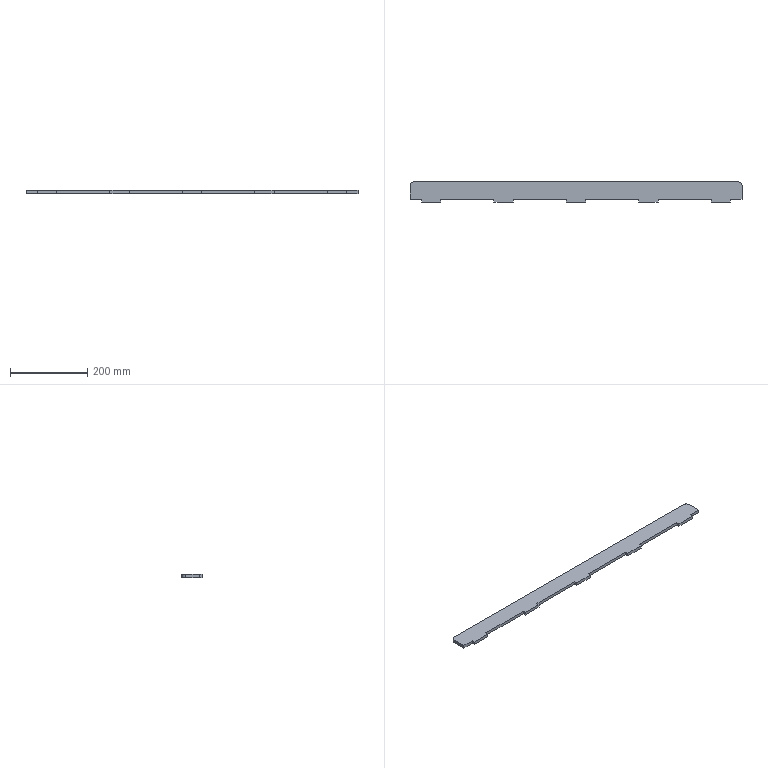Part | SolidWorks | features FlatPattern 1, SMBaseFlange 1, SheetMetal 1 | 1 solid | 28 faces | box 860 x 52.5 x 8 mm | volume 324257 mm3 | plane 26 | cylinder 2 | commonest cylinder face diameters 20 x2
STEP:
#1=CARTESIAN_POINT('',(438.717,-866.,0.));
#2=VERTEX_POINT('',#1);
#3=CARTESIAN_POINT('',(438.717,-831.,0.));
#4=VERTEX_POINT('',#3);
#5=CARTESIAN_POINT('',(438.717,-866.,0.));
#6=DIRECTION('',(0.,1.,0.));
#7=VECTOR('',#6,1000.);
#8=LINE('',#5,#7);
#9=EDGE_CURVE('',#2,#4,#8,.T.);
#10=ORIENTED_EDGE('',*,*,#9,.F.);
#11=CARTESIAN_POINT('',(438.717,-866.,-8.));
#12=VERTEX_POINT('',#11);
#13=CARTESIAN_POINT('',(438.717,-866.,-8.));
#14=DIRECTION('',(0.,0.,1.));
#15=VECTOR('',#14,1000.);
#16=LINE('',#13,#15);
#17=EDGE_CURVE('',#12,#2,#16,.T.);
#18=ORIENTED_EDGE('',*,*,#17,.F.);
#19=CARTESIAN_POINT('',(438.717,-831.,-8.));
#20=VERTEX_POINT('',#19);
#21=CARTESIAN_POINT('',(438.717,-866.,-8.));
#22=DIRECTION('',(0.,1.,0.));
#23=VECTOR('',#22,1000.);
#24=LINE('',#21,#23);
#25=EDGE_CURVE('',#12,#20,#24,.T.);
#26=ORIENTED_EDGE('',*,*,#25,.T.);
#27=CARTESIAN_POINT('',(438.717,-831.,-8.));
#28=DIRECTION('',(0.,0.,1.));
#29=VECTOR('',#28,1000.);
#30=LINE('',#27,#29);
#31=EDGE_CURVE('',#20,#4,#30,.T.);
#32=ORIENTED_EDGE('',*,*,#31,.T.);
#33=EDGE_LOOP('',(#10,#18,#26,#32));
#34=FACE_OUTER_BOUND('',#33,.T.);
#35=CARTESIAN_POINT('',(438.717,-866.,-8.));
#36=DIRECTION('',(1.,0.,0.));
#37=DIRECTION('',(0.,0.,-1.));
#38=AXIS2_PLACEMENT_3D('',#35,#36,#37);
#39=PLANE('',#38);
#40=ADVANCED_FACE('',(#34),#39,.T.);
#41=CARTESIAN_POINT('',(408.717,-866.,0.));
#42=VERTEX_POINT('',#41);
#43=CARTESIAN_POINT('',(438.717,-866.,0.));
#44=DIRECTION('',(1.,0.,0.));
#45=VECTOR('',#44,1000.);
#46=LINE('',#43,#45);
#47=EDGE_CURVE('',#42,#2,#46,.T.);
#48=ORIENTED_EDGE('',*,*,#47,.F.);
#49=CARTESIAN_POINT('',(408.717,-866.,-8.));
#50=VERTEX_POINT('',#49);
#51=CARTESIAN_POINT('',(408.717,-866.,-8.));
#52=DIRECTION('',(0.,0.,1.));
#53=VECTOR('',#52,1000.);
#54=LINE('',#51,#53);
#55=EDGE_CURVE('',#50,#42,#54,.T.);
#56=ORIENTED_EDGE('',*,*,#55,.F.);
#57=CARTESIAN_POINT('',(438.717,-866.,-8.));
#58=DIRECTION('',(1.,0.,0.));
#59=VECTOR('',#58,1000.);
#60=LINE('',#57,#59);
#61=EDGE_CURVE('',#50,#12,#60,.T.);
#62=ORIENTED_EDGE('',*,*,#61,.T.);
#63=ORIENTED_EDGE('',*,*,#17,.T.);
#64=EDGE_LOOP('',(#48,#56,#62,#63));
#65=FACE_OUTER_BOUND('',#64,.T.);
#66=CARTESIAN_POINT('',(438.717,-866.,-8.));
#67=DIRECTION('',(0.,-1.,0.));
#68=DIRECTION('',(0.,0.,-1.));
#69=AXIS2_PLACEMENT_3D('',#66,#67,#68);
#70=PLANE('',#69);
#71=ADVANCED_FACE('',(#65),#70,.T.);
#72=CARTESIAN_POINT('',(408.717,-873.5,0.));
#73=VERTEX_POINT('',#72);
#74=CARTESIAN_POINT('',(408.717,-866.,0.));
#75=DIRECTION('',(0.,1.,0.));
#76=VECTOR('',#75,1000.);
#77=LINE('',#74,#76);
#78=EDGE_CURVE('',#73,#42,#77,.T.);
#79=ORIENTED_EDGE('',*,*,#78,.F.);
#80=CARTESIAN_POINT('',(408.717,-873.5,-8.));
#81=VERTEX_POINT('',#80);
#82=CARTESIAN_POINT('',(408.717,-873.5,-8.));
#83=DIRECTION('',(0.,0.,1.));
#84=VECTOR('',#83,1000.);
#85=LINE('',#82,#84);
#86=EDGE_CURVE('',#81,#73,#85,.T.);
#87=ORIENTED_EDGE('',*,*,#86,.F.);
#88=CARTESIAN_POINT('',(408.717,-866.,-8.));
#89=DIRECTION('',(0.,1.,0.));
#90=VECTOR('',#89,1000.);
#91=LINE('',#88,#90);
#92=EDGE_CURVE('',#81,#50,#91,.T.);
#93=ORIENTED_EDGE('',*,*,#92,.T.);
#94=ORIENTED_EDGE('',*,*,#55,.T.);
#95=EDGE_LOOP('',(#79,#87,#93,#94));
#96=FACE_OUTER_BOUND('',#95,.T.);
#97=CARTESIAN_POINT('',(408.717,-866.,-8.));
#98=DIRECTION('',(1.,0.,0.));
#99=DIRECTION('',(0.,0.,-1.));
#100=AXIS2_PLACEMENT_3D('',#97,#98,#99);
#101=PLANE('',#100);
#102=ADVANCED_FACE('',(#96),#101,.T.);
#103=CARTESIAN_POINT('',(358.717,-873.5,0.));
#104=VERTEX_POINT('',#103);
#105=CARTESIAN_POINT('',(408.717,-873.5,0.));
#106=DIRECTION('',(1.,0.,0.));
#107=VECTOR('',#106,1000.);
#108=LINE('',#105,#107);
#109=EDGE_CURVE('',#104,#73,#108,.T.);
#110=ORIENTED_EDGE('',*,*,#109,.F.);
#111=CARTESIAN_POINT('',(358.717,-873.5,-8.));
#112=VERTEX_POINT('',#111);
#113=CARTESIAN_POINT('',(358.717,-873.5,-8.));
#114=DIRECTION('',(0.,0.,1.));
#115=VECTOR('',#114,1000.);
#116=LINE('',#113,#115);
#117=EDGE_CURVE('',#112,#104,#116,.T.);
#118=ORIENTED_EDGE('',*,*,#117,.F.);
#119=CARTESIAN_POINT('',(408.717,-873.5,-8.));
#120=DIRECTION('',(1.,0.,0.));
#121=VECTOR('',#120,1000.);
#122=LINE('',#119,#121);
#123=EDGE_CURVE('',#112,#81,#122,.T.);
#124=ORIENTED_EDGE('',*,*,#123,.T.);
#125=ORIENTED_EDGE('',*,*,#86,.T.);
#126=EDGE_LOOP('',(#110,#118,#124,#125));
#127=FACE_OUTER_BOUND('',#126,.T.);
#128=CARTESIAN_POINT('',(408.717,-873.5,-8.));
#129=DIRECTION('',(0.,-1.,0.));
#130=DIRECTION('',(0.,0.,-1.));
#131=AXIS2_PLACEMENT_3D('',#128,#129,#130);
#132=PLANE('',#131);
#133=ADVANCED_FACE('',(#127),#132,.T.);
#134=CARTESIAN_POINT('',(358.717,-866.,0.));
#135=VERTEX_POINT('',#134);
#136=CARTESIAN_POINT('',(358.717,-873.5,0.));
#137=DIRECTION('',(0.,-1.,0.));
#138=VECTOR('',#137,1000.);
#139=LINE('',#136,#138);
#140=EDGE_CURVE('',#135,#104,#139,.T.);
#141=ORIENTED_EDGE('',*,*,#140,.F.);
#142=CARTESIAN_POINT('',(358.717,-866.,-8.));
#143=VERTEX_POINT('',#142);
#144=CARTESIAN_POINT('',(358.717,-866.,-8.));
#145=DIRECTION('',(0.,0.,1.));
#146=VECTOR('',#145,1000.);
#147=LINE('',#144,#146);
#148=EDGE_CURVE('',#143,#135,#147,.T.);
#149=ORIENTED_EDGE('',*,*,#148,.F.);
#150=CARTESIAN_POINT('',(358.717,-873.5,-8.));
#151=DIRECTION('',(0.,-1.,0.));
#152=VECTOR('',#151,1000.);
#153=LINE('',#150,#152);
#154=EDGE_CURVE('',#143,#112,#153,.T.);
#155=ORIENTED_EDGE('',*,*,#154,.T.);
#156=ORIENTED_EDGE('',*,*,#117,.T.);
#157=EDGE_LOOP('',(#141,#149,#155,#156));
#158=FACE_OUTER_BOUND('',#157,.T.);
#159=CARTESIAN_POINT('',(358.717,-873.5,-8.));
#160=DIRECTION('',(-1.,0.,0.));
#161=DIRECTION('',(0.,0.,1.));
#162=AXIS2_PLACEMENT_3D('',#159,#160,#161);
#163=PLANE('',#162);
#164=ADVANCED_FACE('',(#158),#163,.T.);
#165=CARTESIAN_POINT('',(221.217,-866.,0.));
#166=VERTEX_POINT('',#165);
#167=CARTESIAN_POINT('',(358.717,-866.,0.));
#168=DIRECTION('',(1.,0.,0.));
#169=VECTOR('',#168,1000.);
#170=LINE('',#167,#169);
#171=EDGE_CURVE('',#166,#135,#170,.T.);
#172=ORIENTED_EDGE('',*,*,#171,.F.);
#173=CARTESIAN_POINT('',(221.217,-866.,-8.));
#174=VERTEX_POINT('',#173);
#175=CARTESIAN_POINT('',(221.217,-866.,-8.));
#176=DIRECTION('',(0.,0.,1.));
#177=VECTOR('',#176,1000.);
#178=LINE('',#175,#177);
#179=EDGE_CURVE('',#174,#166,#178,.T.);
#180=ORIENTED_EDGE('',*,*,#179,.F.);
#181=CARTESIAN_POINT('',(358.717,-866.,-8.));
#182=DIRECTION('',(1.,0.,0.));
#183=VECTOR('',#182,1000.);
#184=LINE('',#181,#183);
#185=EDGE_CURVE('',#174,#143,#184,.T.);
#186=ORIENTED_EDGE('',*,*,#185,.T.);
#187=ORIENTED_EDGE('',*,*,#148,.T.);
#188=EDGE_LOOP('',(#172,#180,#186,#187));
#189=FACE_OUTER_BOUND('',#188,.T.);
#190=CARTESIAN_POINT('',(358.717,-866.,-8.));
#191=DIRECTION('',(0.,-1.,0.));
#192=DIRECTION('',(1.,0.,0.));
#193=AXIS2_PLACEMENT_3D('',#190,#191,#192);
#194=PLANE('',#193);
#195=ADVANCED_FACE('',(#189),#194,.T.);
#196=CARTESIAN_POINT('',(221.217,-873.5,0.));
#197=VERTEX_POINT('',#196);
#198=CARTESIAN_POINT('',(221.217,-866.,0.));
#199=DIRECTION('',(0.,1.,0.));
#200=VECTOR('',#199,1000.);
#201=LINE('',#198,#200);
#202=EDGE_CURVE('',#197,#166,#201,.T.);
#203=ORIENTED_EDGE('',*,*,#202,.F.);
#204=CARTESIAN_POINT('',(221.217,-873.5,-8.));
#205=VERTEX_POINT('',#204);
#206=CARTESIAN_POINT('',(221.217,-873.5,-8.));
#207=DIRECTION('',(0.,0.,1.));
#208=VECTOR('',#207,1000.);
#209=LINE('',#206,#208);
#210=EDGE_CURVE('',#205,#197,#209,.T.);
#211=ORIENTED_EDGE('',*,*,#210,.F.);
#212=CARTESIAN_POINT('',(221.217,-866.,-8.));
#213=DIRECTION('',(0.,1.,0.));
#214=VECTOR('',#213,1000.);
#215=LINE('',#212,#214);
#216=EDGE_CURVE('',#205,#174,#215,.T.);
#217=ORIENTED_EDGE('',*,*,#216,.T.);
#218=ORIENTED_EDGE('',*,*,#179,.T.);
#219=EDGE_LOOP('',(#203,#211,#217,#218));
#220=FACE_OUTER_BOUND('',#219,.T.);
#221=CARTESIAN_POINT('',(221.217,-866.,-8.));
#222=DIRECTION('',(1.,0.,0.));
#223=DIRECTION('',(0.,0.,-1.));
#224=AXIS2_PLACEMENT_3D('',#221,#222,#223);
#225=PLANE('',#224);
#226=ADVANCED_FACE('',(#220),#225,.T.);
#227=CARTESIAN_POINT('',(171.217,-873.5,0.));
#228=VERTEX_POINT('',#227);
#229=CARTESIAN_POINT('',(221.217,-873.5,0.));
#230=DIRECTION('',(1.,0.,0.));
#231=VECTOR('',#230,1000.);
#232=LINE('',#229,#231);
#233=EDGE_CURVE('',#228,#197,#232,.T.);
#234=ORIENTED_EDGE('',*,*,#233,.F.);
#235=CARTESIAN_POINT('',(171.217,-873.5,-8.));
#236=VERTEX_POINT('',#235);
#237=CARTESIAN_POINT('',(171.217,-873.5,-8.));
#238=DIRECTION('',(0.,0.,1.));
#239=VECTOR('',#238,1000.);
#240=LINE('',#237,#239);
#241=EDGE_CURVE('',#236,#228,#240,.T.);
#242=ORIENTED_EDGE('',*,*,#241,.F.);
#243=CARTESIAN_POINT('',(221.217,-873.5,-8.));
#244=DIRECTION('',(1.,0.,0.));
#245=VECTOR('',#244,1000.);
#246=LINE('',#243,#245);
#247=EDGE_CURVE('',#236,#205,#246,.T.);
#248=ORIENTED_EDGE('',*,*,#247,.T.);
#249=ORIENTED_EDGE('',*,*,#210,.T.);
#250=EDGE_LOOP('',(#234,#242,#248,#249));
#251=FACE_OUTER_BOUND('',#250,.T.);
#252=CARTESIAN_POINT('',(221.217,-873.5,-8.));
#253=DIRECTION('',(0.,-1.,0.));
#254=DIRECTION('',(0.,0.,-1.));
#255=AXIS2_PLACEMENT_3D('',#252,#253,#254);
#256=PLANE('',#255);
#257=ADVANCED_FACE('',(#251),#256,.T.);
#258=CARTESIAN_POINT('',(171.217,-866.,0.));
#259=VERTEX_POINT('',#258);
#260=CARTESIAN_POINT('',(171.217,-873.5,0.));
#261=DIRECTION('',(0.,-1.,0.));
#262=VECTOR('',#261,1000.);
#263=LINE('',#260,#262);
#264=EDGE_CURVE('',#259,#228,#263,.T.);
#265=ORIENTED_EDGE('',*,*,#264,.F.);
#266=CARTESIAN_POINT('',(171.217,-866.,-8.));
#267=VERTEX_POINT('',#266);
#268=CARTESIAN_POINT('',(171.217,-866.,-8.));
#269=DIRECTION('',(0.,0.,1.));
#270=VECTOR('',#269,1000.);
#271=LINE('',#268,#270);
#272=EDGE_CURVE('',#267,#259,#271,.T.);
#273=ORIENTED_EDGE('',*,*,#272,.F.);
#274=CARTESIAN_POINT('',(171.217,-873.5,-8.));
#275=DIRECTION('',(0.,-1.,0.));
#276=VECTOR('',#275,1000.);
#277=LINE('',#274,#276);
#278=EDGE_CURVE('',#267,#236,#277,.T.);
#279=ORIENTED_EDGE('',*,*,#278,.T.);
#280=ORIENTED_EDGE('',*,*,#241,.T.);
#281=EDGE_LOOP('',(#265,#273,#279,#280));
#282=FACE_OUTER_BOUND('',#281,.T.);
#283=CARTESIAN_POINT('',(171.217,-873.5,-8.));
#284=DIRECTION('',(-1.,0.,0.));
#285=DIRECTION('',(0.,0.,1.));
#286=AXIS2_PLACEMENT_3D('',#283,#284,#285);
#287=PLANE('',#286);
#288=ADVANCED_FACE('',(#282),#287,.T.);
#289=CARTESIAN_POINT('',(33.717,-866.,0.));
#290=VERTEX_POINT('',#289);
#291=CARTESIAN_POINT('',(171.217,-866.,0.));
#292=DIRECTION('',(1.,0.,0.));
#293=VECTOR('',#292,1000.);
#294=LINE('',#291,#293);
#295=EDGE_CURVE('',#290,#259,#294,.T.);
#296=ORIENTED_EDGE('',*,*,#295,.F.);
#297=CARTESIAN_POINT('',(33.717,-866.,-8.));
#298=VERTEX_POINT('',#297);
#299=CARTESIAN_POINT('',(33.717,-866.,-8.));
#300=DIRECTION('',(0.,0.,1.));
#301=VECTOR('',#300,1000.);
#302=LINE('',#299,#301);
#303=EDGE_CURVE('',#298,#290,#302,.T.);
#304=ORIENTED_EDGE('',*,*,#303,.F.);
#305=CARTESIAN_POINT('',(171.217,-866.,-8.));
#306=DIRECTION('',(1.,0.,0.));
#307=VECTOR('',#306,1000.);
#308=LINE('',#305,#307);
#309=EDGE_CURVE('',#298,#267,#308,.T.);
#310=ORIENTED_EDGE('',*,*,#309,.T.);
#311=ORIENTED_EDGE('',*,*,#272,.T.);
#312=EDGE_LOOP('',(#296,#304,#310,#311));
#313=FACE_OUTER_BOUND('',#312,.T.);
#314=CARTESIAN_POINT('',(171.217,-866.,-8.));
#315=DIRECTION('',(0.,-1.,0.));
#316=DIRECTION('',(1.,0.,0.));
#317=AXIS2_PLACEMENT_3D('',#314,#315,#316);
#318=PLANE('',#317);
#319=ADVANCED_FACE('',(#313),#318,.T.);
#320=CARTESIAN_POINT('',(33.717,-873.5,0.));
#321=VERTEX_POINT('',#320);
#322=CARTESIAN_POINT('',(33.717,-866.,0.));
#323=DIRECTION('',(0.,1.,0.));
#324=VECTOR('',#323,1000.);
#325=LINE('',#322,#324);
#326=EDGE_CURVE('',#321,#290,#325,.T.);
#327=ORIENTED_EDGE('',*,*,#326,.F.);
#328=CARTESIAN_POINT('',(33.717,-873.5,-8.));
#329=VERTEX_POINT('',#328);
#330=CARTESIAN_POINT('',(33.717,-873.5,-8.));
#331=DIRECTION('',(0.,0.,1.));
#332=VECTOR('',#331,1000.);
#333=LINE('',#330,#332);
#334=EDGE_CURVE('',#329,#321,#333,.T.);
#335=ORIENTED_EDGE('',*,*,#334,.F.);
#336=CARTESIAN_POINT('',(33.717,-866.,-8.));
#337=DIRECTION('',(0.,1.,0.));
#338=VECTOR('',#337,1000.);
#339=LINE('',#336,#338);
#340=EDGE_CURVE('',#329,#298,#339,.T.);
#341=ORIENTED_EDGE('',*,*,#340,.T.);
#342=ORIENTED_EDGE('',*,*,#303,.T.);
#343=EDGE_LOOP('',(#327,#335,#341,#342));
#344=FACE_OUTER_BOUND('',#343,.T.);
#345=CARTESIAN_POINT('',(33.717,-866.,-8.));
#346=DIRECTION('',(1.,0.,0.));
#347=DIRECTION('',(0.,0.,-1.));
#348=AXIS2_PLACEMENT_3D('',#345,#346,#347);
#349=PLANE('',#348);
#350=ADVANCED_FACE('',(#344),#349,.T.);
#351=CARTESIAN_POINT('',(-16.283,-873.5,0.));
#352=VERTEX_POINT('',#351);
#353=CARTESIAN_POINT('',(33.717,-873.5,0.));
#354=DIRECTION('',(1.,0.,0.));
#355=VECTOR('',#354,1000.);
#356=LINE('',#353,#355);
#357=EDGE_CURVE('',#352,#321,#356,.T.);
#358=ORIENTED_EDGE('',*,*,#357,.F.);
#359=CARTESIAN_POINT('',(-16.283,-873.5,-8.));
#360=VERTEX_POINT('',#359);
#361=CARTESIAN_POINT('',(-16.283,-873.5,-8.));
#362=DIRECTION('',(0.,0.,1.));
#363=VECTOR('',#362,1000.);
#364=LINE('',#361,#363);
#365=EDGE_CURVE('',#360,#352,#364,.T.);
#366=ORIENTED_EDGE('',*,*,#365,.F.);
#367=CARTESIAN_POINT('',(33.717,-873.5,-8.));
#368=DIRECTION('',(1.,0.,0.));
#369=VECTOR('',#368,1000.);
#370=LINE('',#367,#369);
#371=EDGE_CURVE('',#360,#329,#370,.T.);
#372=ORIENTED_EDGE('',*,*,#371,.T.);
#373=ORIENTED_EDGE('',*,*,#334,.T.);
#374=EDGE_LOOP('',(#358,#366,#372,#373));
#375=FACE_OUTER_BOUND('',#374,.T.);
#376=CARTESIAN_POINT('',(33.717,-873.5,-8.));
#377=DIRECTION('',(0.,-1.,0.));
#378=DIRECTION('',(0.,0.,-1.));
#379=AXIS2_PLACEMENT_3D('',#376,#377,#378);
#380=PLANE('',#379);
#381=ADVANCED_FACE('',(#375),#380,.T.);
#382=CARTESIAN_POINT('',(-16.283,-866.,0.));
#383=VERTEX_POINT('',#382);
#384=CARTESIAN_POINT('',(-16.283,-873.5,0.));
#385=DIRECTION('',(0.,-1.,0.));
#386=VECTOR('',#385,1000.);
#387=LINE('',#384,#386);
#388=EDGE_CURVE('',#383,#352,#387,.T.);
#389=ORIENTED_EDGE('',*,*,#388,.F.);
#390=CARTESIAN_POINT('',(-16.283,-866.,-8.));
#391=VERTEX_POINT('',#390);
#392=CARTESIAN_POINT('',(-16.283,-866.,-8.));
#393=DIRECTION('',(0.,0.,1.));
#394=VECTOR('',#393,1000.);
#395=LINE('',#392,#394);
#396=EDGE_CURVE('',#391,#383,#395,.T.);
#397=ORIENTED_EDGE('',*,*,#396,.F.);
#398=CARTESIAN_POINT('',(-16.283,-873.5,-8.));
#399=DIRECTION('',(0.,-1.,0.));
#400=VECTOR('',#399,1000.);
#401=LINE('',#398,#400);
#402=EDGE_CURVE('',#391,#360,#401,.T.);
#403=ORIENTED_EDGE('',*,*,#402,.T.);
#404=ORIENTED_EDGE('',*,*,#365,.T.);
#405=EDGE_LOOP('',(#389,#397,#403,#404));
#406=FACE_OUTER_BOUND('',#405,.T.);
#407=CARTESIAN_POINT('',(-16.283,-873.5,-8.));
#408=DIRECTION('',(-1.,0.,0.));
#409=DIRECTION('',(0.,0.,1.));
#410=AXIS2_PLACEMENT_3D('',#407,#408,#409);
#411=PLANE('',#410);
#412=ADVANCED_FACE('',(#406),#411,.T.);
#413=CARTESIAN_POINT('',(-153.783,-866.,0.));
#414=VERTEX_POINT('',#413);
#415=CARTESIAN_POINT('',(-16.283,-866.,0.));
#416=DIRECTION('',(1.,0.,0.));
#417=VECTOR('',#416,1000.);
#418=LINE('',#415,#417);
#419=EDGE_CURVE('',#414,#383,#418,.T.);
#420=ORIENTED_EDGE('',*,*,#419,.F.);
#421=CARTESIAN_POINT('',(-153.783,-866.,-8.));
#422=VERTEX_POINT('',#421);
#423=CARTESIAN_POINT('',(-153.783,-866.,-8.));
#424=DIRECTION('',(0.,0.,1.));
#425=VECTOR('',#424,1000.);
#426=LINE('',#423,#425);
#427=EDGE_CURVE('',#422,#414,#426,.T.);
#428=ORIENTED_EDGE('',*,*,#427,.F.);
#429=CARTESIAN_POINT('',(-16.283,-866.,-8.));
#430=DIRECTION('',(1.,0.,0.));
#431=VECTOR('',#430,1000.);
#432=LINE('',#429,#431);
#433=EDGE_CURVE('',#422,#391,#432,.T.);
#434=ORIENTED_EDGE('',*,*,#433,.T.);
#435=ORIENTED_EDGE('',*,*,#396,.T.);
#436=EDGE_LOOP('',(#420,#428,#434,#435));
#437=FACE_OUTER_BOUND('',#436,.T.);
#438=CARTESIAN_POINT('',(-16.283,-866.,-8.));
#439=DIRECTION('',(0.,-1.,0.));
#440=DIRECTION('',(1.,0.,0.));
#441=AXIS2_PLACEMENT_3D('',#438,#439,#440);
#442=PLANE('',#441);
#443=ADVANCED_FACE('',(#437),#442,.T.);
#444=CARTESIAN_POINT('',(-153.783,-873.5,0.));
#445=VERTEX_POINT('',#444);
#446=CARTESIAN_POINT('',(-153.783,-866.,0.));
#447=DIRECTION('',(0.,1.,0.));
#448=VECTOR('',#447,1000.);
#449=LINE('',#446,#448);
#450=EDGE_CURVE('',#445,#414,#449,.T.);
#451=ORIENTED_EDGE('',*,*,#450,.F.);
#452=CARTESIAN_POINT('',(-153.783,-873.5,-8.));
#453=VERTEX_POINT('',#452);
#454=CARTESIAN_POINT('',(-153.783,-873.5,-8.));
#455=DIRECTION('',(0.,0.,1.));
#456=VECTOR('',#455,1000.);
#457=LINE('',#454,#456);
#458=EDGE_CURVE('',#453,#445,#457,.T.);
#459=ORIENTED_EDGE('',*,*,#458,.F.);
#460=CARTESIAN_POINT('',(-153.783,-866.,-8.));
#461=DIRECTION('',(0.,1.,0.));
#462=VECTOR('',#461,1000.);
#463=LINE('',#460,#462);
#464=EDGE_CURVE('',#453,#422,#463,.T.);
#465=ORIENTED_EDGE('',*,*,#464,.T.);
#466=ORIENTED_EDGE('',*,*,#427,.T.);
#467=EDGE_LOOP('',(#451,#459,#465,#466));
#468=FACE_OUTER_BOUND('',#467,.T.);
#469=CARTESIAN_POINT('',(-153.783,-866.,-8.));
#470=DIRECTION('',(1.,0.,0.));
#471=DIRECTION('',(0.,0.,-1.));
#472=AXIS2_PLACEMENT_3D('',#469,#470,#471);
#473=PLANE('',#472);
#474=ADVANCED_FACE('',(#468),#473,.T.);
#475=CARTESIAN_POINT('',(-203.783,-873.5,0.));
#476=VERTEX_POINT('',#475);
#477=CARTESIAN_POINT('',(-153.783,-873.5,0.));
#478=DIRECTION('',(1.,0.,0.));
#479=VECTOR('',#478,1000.);
#480=LINE('',#477,#479);
#481=EDGE_CURVE('',#476,#445,#480,.T.);
#482=ORIENTED_EDGE('',*,*,#481,.F.);
#483=CARTESIAN_POINT('',(-203.783,-873.5,-8.));
#484=VERTEX_POINT('',#483);
#485=CARTESIAN_POINT('',(-203.783,-873.5,-8.));
#486=DIRECTION('',(0.,0.,1.));
#487=VECTOR('',#486,1000.);
#488=LINE('',#485,#487);
#489=EDGE_CURVE('',#484,#476,#488,.T.);
#490=ORIENTED_EDGE('',*,*,#489,.F.);
#491=CARTESIAN_POINT('',(-153.783,-873.5,-8.));
#492=DIRECTION('',(1.,0.,0.));
#493=VECTOR('',#492,1000.);
#494=LINE('',#491,#493);
#495=EDGE_CURVE('',#484,#453,#494,.T.);
#496=ORIENTED_EDGE('',*,*,#495,.T.);
#497=ORIENTED_EDGE('',*,*,#458,.T.);
#498=EDGE_LOOP('',(#482,#490,#496,#497));
#499=FACE_OUTER_BOUND('',#498,.T.);
#500=CARTESIAN_POINT('',(-153.783,-873.5,-8.));
#501=DIRECTION('',(0.,-1.,0.));
#502=DIRECTION('',(0.,0.,-1.));
#503=AXIS2_PLACEMENT_3D('',#500,#501,#502);
#504=PLANE('',#503);
#505=ADVANCED_FACE('',(#499),#504,.T.);
#506=CARTESIAN_POINT('',(-203.783,-866.,0.));
#507=VERTEX_POINT('',#506);
#508=CARTESIAN_POINT('',(-203.783,-873.5,0.));
#509=DIRECTION('',(0.,-1.,0.));
#510=VECTOR('',#509,1000.);
#511=LINE('',#508,#510);
#512=EDGE_CURVE('',#507,#476,#511,.T.);
#513=ORIENTED_EDGE('',*,*,#512,.F.);
#514=CARTESIAN_POINT('',(-203.783,-866.,-8.));
#515=VERTEX_POINT('',#514);
#516=CARTESIAN_POINT('',(-203.783,-866.,-8.));
#517=DIRECTION('',(0.,0.,1.));
#518=VECTOR('',#517,1000.);
#519=LINE('',#516,#518);
#520=EDGE_CURVE('',#515,#507,#519,.T.);
#521=ORIENTED_EDGE('',*,*,#520,.F.);
#522=CARTESIAN_POINT('',(-203.783,-873.5,-8.));
#523=DIRECTION('',(0.,-1.,0.));
#524=VECTOR('',#523,1000.);
#525=LINE('',#522,#524);
#526=EDGE_CURVE('',#515,#484,#525,.T.);
#527=ORIENTED_EDGE('',*,*,#526,.T.);
#528=ORIENTED_EDGE('',*,*,#489,.T.);
#529=EDGE_LOOP('',(#513,#521,#527,#528));
#530=FACE_OUTER_BOUND('',#529,.T.);
#531=CARTESIAN_POINT('',(-203.783,-873.5,-8.));
#532=DIRECTION('',(-1.,0.,0.));
#533=DIRECTION('',(0.,0.,1.));
#534=AXIS2_PLACEMENT_3D('',#531,#532,#533);
#535=PLANE('',#534);
#536=ADVANCED_FACE('',(#530),#535,.T.);
#537=CARTESIAN_POINT('',(-341.283,-866.,0.));
#538=VERTEX_POINT('',#537);
#539=CARTESIAN_POINT('',(-203.783,-866.,0.));
#540=DIRECTION('',(1.,0.,0.));
#541=VECTOR('',#540,1000.);
#542=LINE('',#539,#541);
#543=EDGE_CURVE('',#538,#507,#542,.T.);
#544=ORIENTED_EDGE('',*,*,#543,.F.);
#545=CARTESIAN_POINT('',(-341.283,-866.,-8.));
#546=VERTEX_POINT('',#545);
#547=CARTESIAN_POINT('',(-341.283,-866.,-8.));
#548=DIRECTION('',(0.,0.,1.));
#549=VECTOR('',#548,1000.);
#550=LINE('',#547,#549);
#551=EDGE_CURVE('',#546,#538,#550,.T.);
#552=ORIENTED_EDGE('',*,*,#551,.F.);
#553=CARTESIAN_POINT('',(-203.783,-866.,-8.));
#554=DIRECTION('',(1.,0.,0.));
#555=VECTOR('',#554,1000.);
#556=LINE('',#553,#555);
#557=EDGE_CURVE('',#546,#515,#556,.T.);
#558=ORIENTED_EDGE('',*,*,#557,.T.);
#559=ORIENTED_EDGE('',*,*,#520,.T.);
#560=EDGE_LOOP('',(#544,#552,#558,#559));
#561=FACE_OUTER_BOUND('',#560,.T.);
#562=CARTESIAN_POINT('',(-203.783,-866.,-8.));
#563=DIRECTION('',(0.,-1.,0.));
#564=DIRECTION('',(1.,0.,0.));
#565=AXIS2_PLACEMENT_3D('',#562,#563,#564);
#566=PLANE('',#565);
#567=ADVANCED_FACE('',(#561),#566,.T.);
#568=CARTESIAN_POINT('',(-341.283,-873.5,0.));
#569=VERTEX_POINT('',#568);
#570=CARTESIAN_POINT('',(-341.283,-866.,0.));
#571=DIRECTION('',(0.,1.,0.));
#572=VECTOR('',#571,1000.);
#573=LINE('',#570,#572);
#574=EDGE_CURVE('',#569,#538,#573,.T.);
#575=ORIENTED_EDGE('',*,*,#574,.F.);
#576=CARTESIAN_POINT('',(-341.283,-873.5,-8.));
#577=VERTEX_POINT('',#576);
#578=CARTESIAN_POINT('',(-341.283,-873.5,-8.));
#579=DIRECTION('',(0.,0.,1.));
#580=VECTOR('',#579,1000.);
#581=LINE('',#578,#580);
#582=EDGE_CURVE('',#577,#569,#581,.T.);
#583=ORIENTED_EDGE('',*,*,#582,.F.);
#584=CARTESIAN_POINT('',(-341.283,-866.,-8.));
#585=DIRECTION('',(0.,1.,0.));
#586=VECTOR('',#585,1000.);
#587=LINE('',#584,#586);
#588=EDGE_CURVE('',#577,#546,#587,.T.);
#589=ORIENTED_EDGE('',*,*,#588,.T.);
#590=ORIENTED_EDGE('',*,*,#551,.T.);
#591=EDGE_LOOP('',(#575,#583,#589,#590));
#592=FACE_OUTER_BOUND('',#591,.T.);
#593=CARTESIAN_POINT('',(-341.283,-866.,-8.));
#594=DIRECTION('',(1.,0.,0.));
#595=DIRECTION('',(0.,0.,-1.));
#596=AXIS2_PLACEMENT_3D('',#593,#594,#595);
#597=PLANE('',#596);
#598=ADVANCED_FACE('',(#592),#597,.T.);
#599=CARTESIAN_POINT('',(-391.283,-873.5,0.));
#600=VERTEX_POINT('',#599);
#601=CARTESIAN_POINT('',(-341.283,-873.5,0.));
#602=DIRECTION('',(1.,0.,0.));
#603=VECTOR('',#602,1000.);
#604=LINE('',#601,#603);
#605=EDGE_CURVE('',#600,#569,#604,.T.);
#606=ORIENTED_EDGE('',*,*,#605,.F.);
#607=CARTESIAN_POINT('',(-391.283,-873.5,-8.));
#608=VERTEX_POINT('',#607);
#609=CARTESIAN_POINT('',(-391.283,-873.5,-8.));
#610=DIRECTION('',(0.,0.,1.));
#611=VECTOR('',#610,1000.);
#612=LINE('',#609,#611);
#613=EDGE_CURVE('',#608,#600,#612,.T.);
#614=ORIENTED_EDGE('',*,*,#613,.F.);
#615=CARTESIAN_POINT('',(-341.283,-873.5,-8.));
#616=DIRECTION('',(1.,0.,0.));
#617=VECTOR('',#616,1000.);
#618=LINE('',#615,#617);
#619=EDGE_CURVE('',#608,#577,#618,.T.);
#620=ORIENTED_EDGE('',*,*,#619,.T.);
#621=ORIENTED_EDGE('',*,*,#582,.T.);
#622=EDGE_LOOP('',(#606,#614,#620,#621));
#623=FACE_OUTER_BOUND('',#622,.T.);
#624=CARTESIAN_POINT('',(-341.283,-873.5,-8.));
#625=DIRECTION('',(0.,-1.,0.));
#626=DIRECTION('',(0.,0.,-1.));
#627=AXIS2_PLACEMENT_3D('',#624,#625,#626);
#628=PLANE('',#627);
#629=ADVANCED_FACE('',(#623),#628,.T.);
#630=CARTESIAN_POINT('',(-391.283,-866.,0.));
#631=VERTEX_POINT('',#630);
#632=CARTESIAN_POINT('',(-391.283,-873.5,0.));
#633=DIRECTION('',(0.,-1.,0.));
#634=VECTOR('',#633,1000.);
#635=LINE('',#632,#634);
#636=EDGE_CURVE('',#631,#600,#635,.T.);
#637=ORIENTED_EDGE('',*,*,#636,.F.);
#638=CARTESIAN_POINT('',(-391.283,-866.,-8.));
#639=VERTEX_POINT('',#638);
#640=CARTESIAN_POINT('',(-391.283,-866.,-8.));
#641=DIRECTION('',(0.,0.,1.));
#642=VECTOR('',#641,1000.);
#643=LINE('',#640,#642);
#644=EDGE_CURVE('',#639,#631,#643,.T.);
#645=ORIENTED_EDGE('',*,*,#644,.F.);
#646=CARTESIAN_POINT('',(-391.283,-873.5,-8.));
#647=DIRECTION('',(0.,-1.,0.));
#648=VECTOR('',#647,1000.);
#649=LINE('',#646,#648);
#650=EDGE_CURVE('',#639,#608,#649,.T.);
#651=ORIENTED_EDGE('',*,*,#650,.T.);
#652=ORIENTED_EDGE('',*,*,#613,.T.);
#653=EDGE_LOOP('',(#637,#645,#651,#652));
#654=FACE_OUTER_BOUND('',#653,.T.);
#655=CARTESIAN_POINT('',(-391.283,-873.5,-8.));
#656=DIRECTION('',(-1.,0.,0.));
#657=DIRECTION('',(0.,0.,1.));
#658=AXIS2_PLACEMENT_3D('',#655,#656,#657);
#659=PLANE('',#658);
#660=ADVANCED_FACE('',(#654),#659,.T.);
#661=CARTESIAN_POINT('',(-421.283,-866.,0.));
#662=VERTEX_POINT('',#661);
#663=CARTESIAN_POINT('',(-391.283,-866.,0.));
#664=DIRECTION('',(1.,0.,0.));
#665=VECTOR('',#664,1000.);
#666=LINE('',#663,#665);
#667=EDGE_CURVE('',#662,#631,#666,.T.);
#668=ORIENTED_EDGE('',*,*,#667,.F.);
#669=CARTESIAN_POINT('',(-421.283,-866.,-8.));
#670=VERTEX_POINT('',#669);
#671=CARTESIAN_POINT('',(-421.283,-866.,-8.));
#672=DIRECTION('',(0.,0.,1.));
#673=VECTOR('',#672,1000.);
#674=LINE('',#671,#673);
#675=EDGE_CURVE('',#670,#662,#674,.T.);
#676=ORIENTED_EDGE('',*,*,#675,.F.);
#677=CARTESIAN_POINT('',(-391.283,-866.,-8.));
#678=DIRECTION('',(1.,0.,0.));
#679=VECTOR('',#678,1000.);
#680=LINE('',#677,#679);
#681=EDGE_CURVE('',#670,#639,#680,.T.);
#682=ORIENTED_EDGE('',*,*,#681,.T.);
#683=ORIENTED_EDGE('',*,*,#644,.T.);
#684=EDGE_LOOP('',(#668,#676,#682,#683));
#685=FACE_OUTER_BOUND('',#684,.T.);
#686=CARTESIAN_POINT('',(-391.283,-866.,-8.));
#687=DIRECTION('',(0.,-1.,0.));
#688=DIRECTION('',(1.,0.,0.));
#689=AXIS2_PLACEMENT_3D('',#686,#687,#688);
#690=PLANE('',#689);
#691=ADVANCED_FACE('',(#685),#690,.T.);
#692=CARTESIAN_POINT('',(-421.283,-831.,0.));
#693=VERTEX_POINT('',#692);
#694=CARTESIAN_POINT('',(-421.283,-866.,0.));
#695=DIRECTION('',(0.,-1.,0.));
#696=VECTOR('',#695,1000.);
#697=LINE('',#694,#696);
#698=EDGE_CURVE('',#693,#662,#697,.T.);
#699=ORIENTED_EDGE('',*,*,#698,.F.);
#700=CARTESIAN_POINT('',(-421.283,-831.,-8.));
#701=VERTEX_POINT('',#700);
#702=CARTESIAN_POINT('',(-421.283,-831.,-8.));
#703=DIRECTION('',(0.,0.,1.));
#704=VECTOR('',#703,1000.);
#705=LINE('',#702,#704);
#706=EDGE_CURVE('',#701,#693,#705,.T.);
#707=ORIENTED_EDGE('',*,*,#706,.F.);
#708=CARTESIAN_POINT('',(-421.283,-866.,-8.));
#709=DIRECTION('',(0.,-1.,0.));
#710=VECTOR('',#709,1000.);
#711=LINE('',#708,#710);
#712=EDGE_CURVE('',#701,#670,#711,.T.);
#713=ORIENTED_EDGE('',*,*,#712,.T.);
#714=ORIENTED_EDGE('',*,*,#675,.T.);
#715=EDGE_LOOP('',(#699,#707,#713,#714));
#716=FACE_OUTER_BOUND('',#715,.T.);
#717=CARTESIAN_POINT('',(-421.283,-866.,-8.));
#718=DIRECTION('',(-1.,0.,0.));
#719=DIRECTION('',(0.,-1.,0.));
#720=AXIS2_PLACEMENT_3D('',#717,#718,#719);
#721=PLANE('',#720);
#722=ADVANCED_FACE('',(#716),#721,.T.);
#723=CARTESIAN_POINT('',(-411.283,-821.,0.));
#724=VERTEX_POINT('',#723);
#725=CARTESIAN_POINT('',(-411.283,-831.,0.));
#726=DIRECTION('',(0.,0.,1.));
#727=DIRECTION('',(1.,0.,0.));
#728=AXIS2_PLACEMENT_3D('',#725,#726,#727);
#729=CIRCLE('',#728,10.);
#730=EDGE_CURVE('',#724,#693,#729,.T.);
#731=ORIENTED_EDGE('',*,*,#730,.F.);
#732=CARTESIAN_POINT('',(-411.283,-821.,-8.));
#733=VERTEX_POINT('',#732);
#734=CARTESIAN_POINT('',(-411.283,-821.,-8.));
#735=DIRECTION('',(0.,0.,1.));
#736=VECTOR('',#735,1000.);
#737=LINE('',#734,#736);
#738=EDGE_CURVE('',#733,#724,#737,.T.);
#739=ORIENTED_EDGE('',*,*,#738,.F.);
#740=CARTESIAN_POINT('',(-411.283,-831.,-8.));
#741=DIRECTION('',(0.,0.,1.));
#742=DIRECTION('',(1.,0.,0.));
#743=AXIS2_PLACEMENT_3D('',#740,#741,#742);
#744=CIRCLE('',#743,10.);
#745=EDGE_CURVE('',#733,#701,#744,.T.);
#746=ORIENTED_EDGE('',*,*,#745,.T.);
#747=ORIENTED_EDGE('',*,*,#706,.T.);
#748=EDGE_LOOP('',(#731,#739,#746,#747));
#749=FACE_OUTER_BOUND('',#748,.T.);
#750=CARTESIAN_POINT('',(-411.283,-831.,-8.));
#751=DIRECTION('',(0.,0.,1.));
#752=DIRECTION('',(1.,0.,0.));
#753=AXIS2_PLACEMENT_3D('',#750,#751,#752);
#754=CYLINDRICAL_SURFACE('',#753,10.);
#755=ADVANCED_FACE('',(#749),#754,.T.);
#756=CARTESIAN_POINT('',(428.717,-821.,0.));
#757=VERTEX_POINT('',#756);
#758=CARTESIAN_POINT('',(428.717,-821.,0.));
#759=DIRECTION('',(-1.,0.,0.));
#760=VECTOR('',#759,1000.);
#761=LINE('',#758,#760);
#762=EDGE_CURVE('',#757,#724,#761,.T.);
#763=ORIENTED_EDGE('',*,*,#762,.F.);
#764=CARTESIAN_POINT('',(428.717,-821.,-8.));
#765=VERTEX_POINT('',#764);
#766=CARTESIAN_POINT('',(428.717,-821.,-8.));
#767=DIRECTION('',(0.,0.,1.));
#768=VECTOR('',#767,1000.);
#769=LINE('',#766,#768);
#770=EDGE_CURVE('',#765,#757,#769,.T.);
#771=ORIENTED_EDGE('',*,*,#770,.F.);
#772=CARTESIAN_POINT('',(428.717,-821.,-8.));
#773=DIRECTION('',(-1.,0.,0.));
#774=VECTOR('',#773,1000.);
#775=LINE('',#772,#774);
#776=EDGE_CURVE('',#765,#733,#775,.T.);
#777=ORIENTED_EDGE('',*,*,#776,.T.);
#778=ORIENTED_EDGE('',*,*,#738,.T.);
#779=EDGE_LOOP('',(#763,#771,#777,#778));
#780=FACE_OUTER_BOUND('',#779,.T.);
#781=CARTESIAN_POINT('',(428.717,-821.,-8.));
#782=DIRECTION('',(0.,1.,0.));
#783=DIRECTION('',(-1.,0.,0.));
#784=AXIS2_PLACEMENT_3D('',#781,#782,#783);
#785=PLANE('',#784);
#786=ADVANCED_FACE('',(#780),#785,.T.);
#787=CARTESIAN_POINT('',(428.717,-831.,0.));
#788=DIRECTION('',(0.,0.,1.));
#789=DIRECTION('',(1.,0.,0.));
#790=AXIS2_PLACEMENT_3D('',#787,#788,#789);
#791=CIRCLE('',#790,10.);
#792=EDGE_CURVE('',#4,#757,#791,.T.);
#793=ORIENTED_EDGE('',*,*,#792,.F.);
#794=ORIENTED_EDGE('',*,*,#31,.F.);
#795=CARTESIAN_POINT('',(428.717,-831.,-8.));
#796=DIRECTION('',(0.,0.,1.));
#797=DIRECTION('',(1.,0.,0.));
#798=AXIS2_PLACEMENT_3D('',#795,#796,#797);
#799=CIRCLE('',#798,10.);
#800=EDGE_CURVE('',#20,#765,#799,.T.);
#801=ORIENTED_EDGE('',*,*,#800,.T.);
#802=ORIENTED_EDGE('',*,*,#770,.T.);
#803=EDGE_LOOP('',(#793,#794,#801,#802));
#804=FACE_OUTER_BOUND('',#803,.T.);
#805=CARTESIAN_POINT('',(428.717,-831.,-8.));
#806=DIRECTION('',(0.,0.,1.));
#807=DIRECTION('',(1.,0.,0.));
#808=AXIS2_PLACEMENT_3D('',#805,#806,#807);
#809=CYLINDRICAL_SURFACE('',#808,10.);
#810=ADVANCED_FACE('',(#804),#809,.T.);
#811=ORIENTED_EDGE('',*,*,#25,.F.);
#812=ORIENTED_EDGE('',*,*,#61,.F.);
#813=ORIENTED_EDGE('',*,*,#92,.F.);
#814=ORIENTED_EDGE('',*,*,#123,.F.);
#815=ORIENTED_EDGE('',*,*,#154,.F.);
#816=ORIENTED_EDGE('',*,*,#185,.F.);
#817=ORIENTED_EDGE('',*,*,#216,.F.);
#818=ORIENTED_EDGE('',*,*,#247,.F.);
#819=ORIENTED_EDGE('',*,*,#278,.F.);
#820=ORIENTED_EDGE('',*,*,#309,.F.);
#821=ORIENTED_EDGE('',*,*,#340,.F.);
#822=ORIENTED_EDGE('',*,*,#371,.F.);
#823=ORIENTED_EDGE('',*,*,#402,.F.);
#824=ORIENTED_EDGE('',*,*,#433,.F.);
#825=ORIENTED_EDGE('',*,*,#464,.F.);
#826=ORIENTED_EDGE('',*,*,#495,.F.);
#827=ORIENTED_EDGE('',*,*,#526,.F.);
#828=ORIENTED_EDGE('',*,*,#557,.F.);
#829=ORIENTED_EDGE('',*,*,#588,.F.);
#830=ORIENTED_EDGE('',*,*,#619,.F.);
#831=ORIENTED_EDGE('',*,*,#650,.F.);
#832=ORIENTED_EDGE('',*,*,#681,.F.);
#833=ORIENTED_EDGE('',*,*,#712,.F.);
#834=ORIENTED_EDGE('',*,*,#745,.F.);
#835=ORIENTED_EDGE('',*,*,#776,.F.);
#836=ORIENTED_EDGE('',*,*,#800,.F.);
#837=EDGE_LOOP('',(#811,#812,#813,#814,#815,#816,#817,#818,#819,#820,#821,#822,#823,#824,#825,#826,#827,#828,#829,#830,#831,#832,#833,#834,#835,#836));
#838=FACE_OUTER_BOUND('',#837,.T.);
#839=CARTESIAN_POINT('',(428.717,-831.,-8.));
#840=DIRECTION('',(0.,0.,1.));
#841=DIRECTION('',(1.,0.,0.));
#842=AXIS2_PLACEMENT_3D('',#839,#840,#841);
#843=PLANE('',#842);
#844=ADVANCED_FACE('',(#838),#843,.F.);
#845=ORIENTED_EDGE('',*,*,#9,.T.);
#846=ORIENTED_EDGE('',*,*,#792,.T.);
#847=ORIENTED_EDGE('',*,*,#762,.T.);
#848=ORIENTED_EDGE('',*,*,#730,.T.);
#849=ORIENTED_EDGE('',*,*,#698,.T.);
#850=ORIENTED_EDGE('',*,*,#667,.T.);
#851=ORIENTED_EDGE('',*,*,#636,.T.);
#852=ORIENTED_EDGE('',*,*,#605,.T.);
#853=ORIENTED_EDGE('',*,*,#574,.T.);
#854=ORIENTED_EDGE('',*,*,#543,.T.);
#855=ORIENTED_EDGE('',*,*,#512,.T.);
#856=ORIENTED_EDGE('',*,*,#481,.T.);
#857=ORIENTED_EDGE('',*,*,#450,.T.);
#858=ORIENTED_EDGE('',*,*,#419,.T.);
#859=ORIENTED_EDGE('',*,*,#388,.T.);
#860=ORIENTED_EDGE('',*,*,#357,.T.);
#861=ORIENTED_EDGE('',*,*,#326,.T.);
#862=ORIENTED_EDGE('',*,*,#295,.T.);
#863=ORIENTED_EDGE('',*,*,#264,.T.);
#864=ORIENTED_EDGE('',*,*,#233,.T.);
#865=ORIENTED_EDGE('',*,*,#202,.T.);
#866=ORIENTED_EDGE('',*,*,#171,.T.);
#867=ORIENTED_EDGE('',*,*,#140,.T.);
#868=ORIENTED_EDGE('',*,*,#109,.T.);
#869=ORIENTED_EDGE('',*,*,#78,.T.);
#870=ORIENTED_EDGE('',*,*,#47,.T.);
#871=EDGE_LOOP('',(#845,#846,#847,#848,#849,#850,#851,#852,#853,#854,#855,#856,#857,#858,#859,#860,#861,#862,#863,#864,#865,#866,#867,#868,#869,#870));
#872=FACE_OUTER_BOUND('',#871,.T.);
#873=CARTESIAN_POINT('',(428.717,-831.,0.));
#874=DIRECTION('',(0.,0.,1.));
#875=DIRECTION('',(1.,0.,0.));
#876=AXIS2_PLACEMENT_3D('',#873,#874,#875);
#877=PLANE('',#876);
#878=ADVANCED_FACE('',(#872),#877,.T.);
#879=CLOSED_SHELL('',(#40,#71,#102,#133,#164,#195,#226,#257,#288,#319,#350,#381,#412,#443,#474,#505,#536,#567,#598,#629,#660,#691,#722,#755,#786,#810,#844,#878));
#880=MANIFOLD_SOLID_BREP('',#879);
#881=CARTESIAN_POINT('',(0.,0.,0.));
#882=DIRECTION('',(0.,0.,1.));
#883=DIRECTION('',(1.,0.,0.));
#884=AXIS2_PLACEMENT_3D('',#881,#882,#883);
#885=(LENGTH_UNIT()NAMED_UNIT(*)SI_UNIT(.MILLI.,.METRE.));
#886=UNCERTAINTY_MEASURE_WITH_UNIT(LENGTH_MEASURE(0.00001),#885,'','');
#887=(NAMED_UNIT(*)PLANE_ANGLE_UNIT()SI_UNIT($,.RADIAN.));
#888=(NAMED_UNIT(*)SI_UNIT($,.STERADIAN.)SOLID_ANGLE_UNIT());
#889=(GEOMETRIC_REPRESENTATION_CONTEXT(3)GLOBAL_UNCERTAINTY_ASSIGNED_CONTEXT((#886))GLOBAL_UNIT_ASSIGNED_CONTEXT((#885,#887,#888))REPRESENTATION_CONTEXT('',''));
#890=ADVANCED_BREP_SHAPE_REPRESENTATION('',(#880,#884),#889);